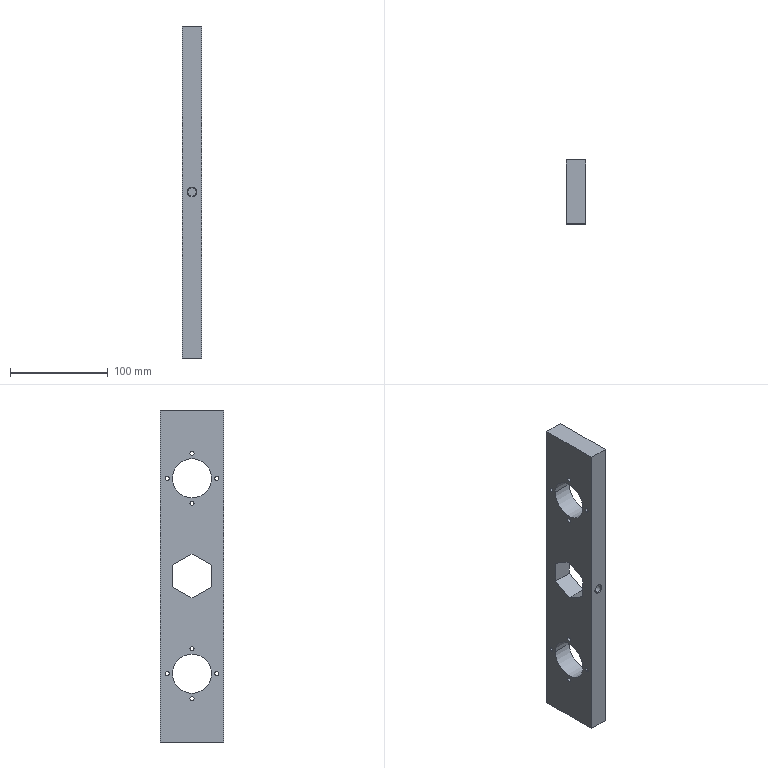Part | STEP file | 1 solid | 60 faces | box 20 x 65 x 340 mm | volume 355958 mm3 | cylinder 30 | cone 18 | plane 12 | commonest cylinder face diameters 4.2 x16 8.5 x10 40 x4